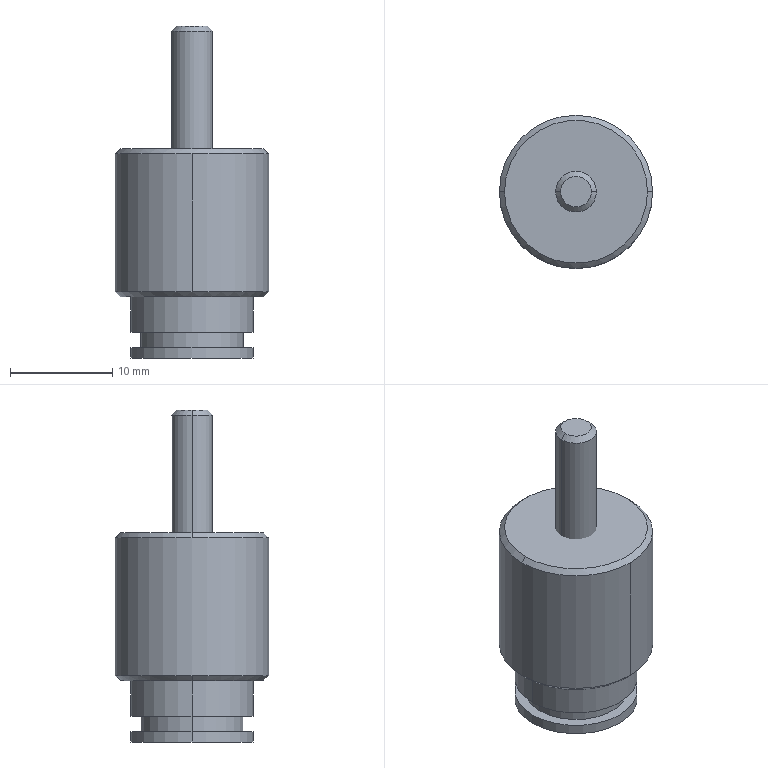Part | STEP file | Cylinder CCOMPANY_AB 10-5_Retract | 2 solids | 26 faces | box 15 x 15 x 32.5 mm | volume 3211 mm3 | cylinder 12 | plane 8 | cone 6 | commonest cylinder face diameters 12 x4 4 x2 8.2 x2 10 x2 15 x2